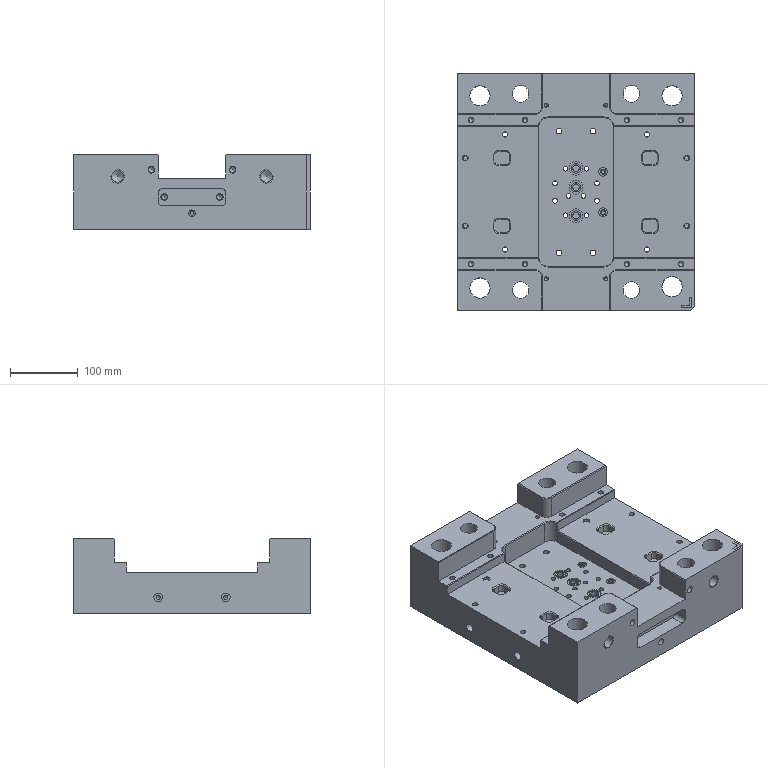Part | NX | features BB 2 | 1 solid | 437 faces | box 350 x 350 x 110 mm | volume 7497373 mm3 | plane 183 | cylinder 178 | cone 76 | commonest cylinder face diameters 12 x28 6 x18 8 x14 8.5 x12 10 x12 7 x10